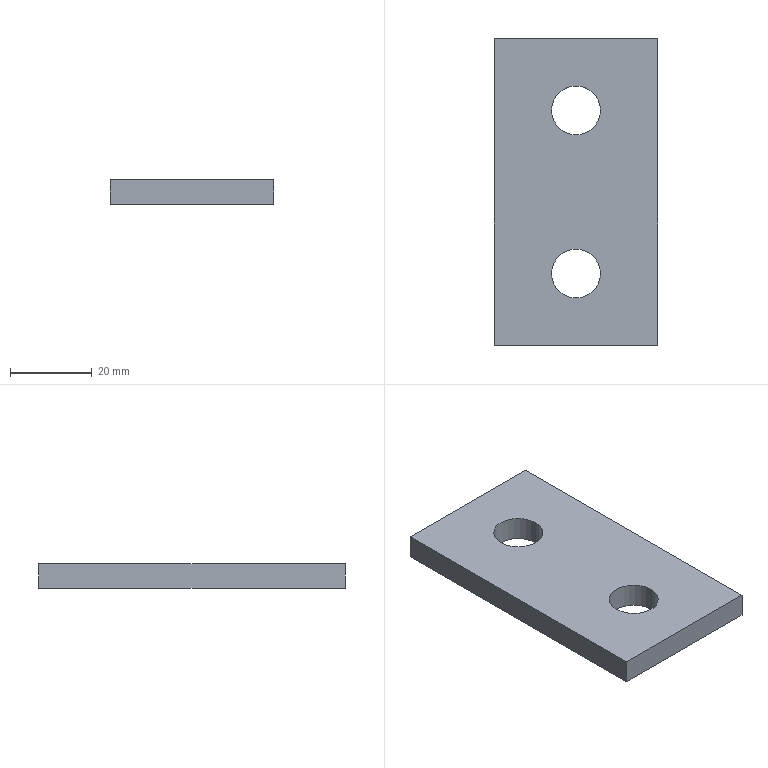Part | STEP file | BCC3 H13_10 | 1 solid | 10 faces | box 40 x 75 x 6 mm | volume 16643 mm3 | plane 6 | cylinder 4 | commonest cylinder face diameters 12 x4
STEP:
#1=CARTESIAN_POINT('',(0.,0.,0.));
#2=DIRECTION('',(0.,0.,1.));
#3=DIRECTION('',(1.,0.,0.));
#4=AXIS2_PLACEMENT_3D('',#1,#2,#3);
#5=CARTESIAN_POINT('',(6.,-20.,0.));
#6=VERTEX_POINT('',#5);
#7=CARTESIAN_POINT('',(6.,-20.,6.));
#8=VERTEX_POINT('',#7);
#9=CARTESIAN_POINT('',(6.,-20.,0.));
#10=DIRECTION('',(0.,0.,1.));
#11=VECTOR('',#10,1.);
#12=LINE('',#9,#11);
#13=CARTESIAN_POINT('',(0.,-20.,0.));
#14=DIRECTION('',(0.,0.,1.));
#15=DIRECTION('',(1.,0.,0.));
#16=AXIS2_PLACEMENT_3D('',#13,#14,#15);
#17=CYLINDRICAL_SURFACE('',#16,6.);
#18=CARTESIAN_POINT('',(6.283,0.));
#19=DIRECTION('',(0.,1.));
#20=VECTOR('',#19,1.);
#21=LINE('',#18,#20);
#22=(GEOMETRIC_REPRESENTATION_CONTEXT(2)PARAMETRIC_REPRESENTATION_CONTEXT()REPRESENTATION_CONTEXT('',''));
#23=DEFINITIONAL_REPRESENTATION('',(#21),#22);
#24=PCURVE('',#17,#23);
#25=CARTESIAN_POINT('',(0.,-20.,0.));
#26=DIRECTION('',(0.,0.,1.));
#27=DIRECTION('',(1.,0.,0.));
#28=AXIS2_PLACEMENT_3D('',#25,#26,#27);
#29=CYLINDRICAL_SURFACE('',#28,6.);
#30=CARTESIAN_POINT('',(0.,0.));
#31=DIRECTION('',(0.,1.));
#32=VECTOR('',#31,1.);
#33=LINE('',#30,#32);
#34=(GEOMETRIC_REPRESENTATION_CONTEXT(2)PARAMETRIC_REPRESENTATION_CONTEXT()REPRESENTATION_CONTEXT('',''));
#35=DEFINITIONAL_REPRESENTATION('',(#33),#34);
#36=PCURVE('',#29,#35);
#37=SURFACE_CURVE('',#12,(#24,#36),.PCURVE_S1.);
#38=EDGE_CURVE('',#6,#8,#37,.T.);
#39=ORIENTED_EDGE('',*,*,#38,.T.);
#40=CARTESIAN_POINT('',(-6.,-20.,6.));
#41=VERTEX_POINT('',#40);
#42=CARTESIAN_POINT('',(0.,-20.,6.));
#43=DIRECTION('',(0.,0.,1.));
#44=DIRECTION('',(1.,0.,0.));
#45=AXIS2_PLACEMENT_3D('',#42,#43,#44);
#46=CIRCLE('',#45,6.);
#47=CARTESIAN_POINT('',(0.,6.));
#48=DIRECTION('',(1.,0.));
#49=VECTOR('',#48,1.);
#50=LINE('',#47,#49);
#51=(GEOMETRIC_REPRESENTATION_CONTEXT(2)PARAMETRIC_REPRESENTATION_CONTEXT()REPRESENTATION_CONTEXT('',''));
#52=DEFINITIONAL_REPRESENTATION('',(#50),#51);
#53=PCURVE('',#17,#52);
#54=CARTESIAN_POINT('',(0.,0.,6.));
#55=DIRECTION('',(0.,0.,1.));
#56=DIRECTION('',(1.,0.,0.));
#57=AXIS2_PLACEMENT_3D('',#54,#55,#56);
#58=PLANE('',#57);
#59=CARTESIAN_POINT('',(0.,-20.));
#60=DIRECTION('',(1.,0.));
#61=AXIS2_PLACEMENT_2D('',#59,#60);
#62=CIRCLE('',#61,6.);
#63=(GEOMETRIC_REPRESENTATION_CONTEXT(2)PARAMETRIC_REPRESENTATION_CONTEXT()REPRESENTATION_CONTEXT('',''));
#64=DEFINITIONAL_REPRESENTATION('',(#62),#63);
#65=PCURVE('',#58,#64);
#66=SURFACE_CURVE('',#46,(#53,#65),.PCURVE_S1.);
#67=EDGE_CURVE('',#41,#8,#66,.T.);
#68=ORIENTED_EDGE('',*,*,#67,.F.);
#69=CARTESIAN_POINT('',(-6.,-20.,0.));
#70=VERTEX_POINT('',#69);
#71=CARTESIAN_POINT('',(-6.,-20.,0.));
#72=DIRECTION('',(0.,0.,1.));
#73=VECTOR('',#72,1.);
#74=LINE('',#71,#73);
#75=CARTESIAN_POINT('',(3.142,0.));
#76=DIRECTION('',(0.,1.));
#77=VECTOR('',#76,1.);
#78=LINE('',#75,#77);
#79=(GEOMETRIC_REPRESENTATION_CONTEXT(2)PARAMETRIC_REPRESENTATION_CONTEXT()REPRESENTATION_CONTEXT('',''));
#80=DEFINITIONAL_REPRESENTATION('',(#78),#79);
#81=PCURVE('',#17,#80);
#82=CARTESIAN_POINT('',(3.142,0.));
#83=DIRECTION('',(0.,1.));
#84=VECTOR('',#83,1.);
#85=LINE('',#82,#84);
#86=(GEOMETRIC_REPRESENTATION_CONTEXT(2)PARAMETRIC_REPRESENTATION_CONTEXT()REPRESENTATION_CONTEXT('',''));
#87=DEFINITIONAL_REPRESENTATION('',(#85),#86);
#88=PCURVE('',#29,#87);
#89=SURFACE_CURVE('',#74,(#81,#88),.PCURVE_S1.);
#90=EDGE_CURVE('',#70,#41,#89,.T.);
#91=ORIENTED_EDGE('',*,*,#90,.F.);
#92=CARTESIAN_POINT('',(0.,-20.,0.));
#93=DIRECTION('',(0.,0.,1.));
#94=DIRECTION('',(1.,0.,0.));
#95=AXIS2_PLACEMENT_3D('',#92,#93,#94);
#96=CIRCLE('',#95,6.);
#97=CARTESIAN_POINT('',(0.,0.));
#98=DIRECTION('',(1.,0.));
#99=VECTOR('',#98,1.);
#100=LINE('',#97,#99);
#101=(GEOMETRIC_REPRESENTATION_CONTEXT(2)PARAMETRIC_REPRESENTATION_CONTEXT()REPRESENTATION_CONTEXT('',''));
#102=DEFINITIONAL_REPRESENTATION('',(#100),#101);
#103=PCURVE('',#17,#102);
#104=CARTESIAN_POINT('',(0.,0.,0.));
#105=DIRECTION('',(0.,0.,1.));
#106=DIRECTION('',(1.,0.,0.));
#107=AXIS2_PLACEMENT_3D('',#104,#105,#106);
#108=PLANE('',#107);
#109=CARTESIAN_POINT('',(0.,-20.));
#110=DIRECTION('',(1.,0.));
#111=AXIS2_PLACEMENT_2D('',#109,#110);
#112=CIRCLE('',#111,6.);
#113=(GEOMETRIC_REPRESENTATION_CONTEXT(2)PARAMETRIC_REPRESENTATION_CONTEXT()REPRESENTATION_CONTEXT('',''));
#114=DEFINITIONAL_REPRESENTATION('',(#112),#113);
#115=PCURVE('',#108,#114);
#116=SURFACE_CURVE('',#96,(#103,#115),.PCURVE_S1.);
#117=EDGE_CURVE('',#70,#6,#116,.T.);
#118=ORIENTED_EDGE('',*,*,#117,.T.);
#119=EDGE_LOOP('',(#39,#68,#91,#118));
#120=FACE_BOUND('',#119,.F.);
#121=ADVANCED_FACE('',(#120),#17,.F.);
#122=CARTESIAN_POINT('',(6.,20.,0.));
#123=VERTEX_POINT('',#122);
#124=CARTESIAN_POINT('',(6.,20.,6.));
#125=VERTEX_POINT('',#124);
#126=CARTESIAN_POINT('',(6.,20.,0.));
#127=DIRECTION('',(0.,0.,1.));
#128=VECTOR('',#127,1.);
#129=LINE('',#126,#128);
#130=CARTESIAN_POINT('',(0.,20.,0.));
#131=DIRECTION('',(0.,0.,1.));
#132=DIRECTION('',(1.,0.,0.));
#133=AXIS2_PLACEMENT_3D('',#130,#131,#132);
#134=CYLINDRICAL_SURFACE('',#133,6.);
#135=CARTESIAN_POINT('',(6.283,0.));
#136=DIRECTION('',(0.,1.));
#137=VECTOR('',#136,1.);
#138=LINE('',#135,#137);
#139=(GEOMETRIC_REPRESENTATION_CONTEXT(2)PARAMETRIC_REPRESENTATION_CONTEXT()REPRESENTATION_CONTEXT('',''));
#140=DEFINITIONAL_REPRESENTATION('',(#138),#139);
#141=PCURVE('',#134,#140);
#142=CARTESIAN_POINT('',(0.,20.,0.));
#143=DIRECTION('',(0.,0.,1.));
#144=DIRECTION('',(1.,0.,0.));
#145=AXIS2_PLACEMENT_3D('',#142,#143,#144);
#146=CYLINDRICAL_SURFACE('',#145,6.);
#147=CARTESIAN_POINT('',(0.,0.));
#148=DIRECTION('',(0.,1.));
#149=VECTOR('',#148,1.);
#150=LINE('',#147,#149);
#151=(GEOMETRIC_REPRESENTATION_CONTEXT(2)PARAMETRIC_REPRESENTATION_CONTEXT()REPRESENTATION_CONTEXT('',''));
#152=DEFINITIONAL_REPRESENTATION('',(#150),#151);
#153=PCURVE('',#146,#152);
#154=SURFACE_CURVE('',#129,(#141,#153),.PCURVE_S1.);
#155=EDGE_CURVE('',#123,#125,#154,.T.);
#156=ORIENTED_EDGE('',*,*,#155,.T.);
#157=CARTESIAN_POINT('',(-6.,20.,6.));
#158=VERTEX_POINT('',#157);
#159=CARTESIAN_POINT('',(0.,20.,6.));
#160=DIRECTION('',(0.,0.,1.));
#161=DIRECTION('',(1.,0.,0.));
#162=AXIS2_PLACEMENT_3D('',#159,#160,#161);
#163=CIRCLE('',#162,6.);
#164=CARTESIAN_POINT('',(0.,6.));
#165=DIRECTION('',(1.,0.));
#166=VECTOR('',#165,1.);
#167=LINE('',#164,#166);
#168=(GEOMETRIC_REPRESENTATION_CONTEXT(2)PARAMETRIC_REPRESENTATION_CONTEXT()REPRESENTATION_CONTEXT('',''));
#169=DEFINITIONAL_REPRESENTATION('',(#167),#168);
#170=PCURVE('',#134,#169);
#171=CARTESIAN_POINT('',(0.,20.));
#172=DIRECTION('',(1.,0.));
#173=AXIS2_PLACEMENT_2D('',#171,#172);
#174=CIRCLE('',#173,6.);
#175=(GEOMETRIC_REPRESENTATION_CONTEXT(2)PARAMETRIC_REPRESENTATION_CONTEXT()REPRESENTATION_CONTEXT('',''));
#176=DEFINITIONAL_REPRESENTATION('',(#174),#175);
#177=PCURVE('',#58,#176);
#178=SURFACE_CURVE('',#163,(#170,#177),.PCURVE_S1.);
#179=EDGE_CURVE('',#158,#125,#178,.T.);
#180=ORIENTED_EDGE('',*,*,#179,.F.);
#181=CARTESIAN_POINT('',(-6.,20.,0.));
#182=VERTEX_POINT('',#181);
#183=CARTESIAN_POINT('',(-6.,20.,0.));
#184=DIRECTION('',(0.,0.,1.));
#185=VECTOR('',#184,1.);
#186=LINE('',#183,#185);
#187=CARTESIAN_POINT('',(3.142,0.));
#188=DIRECTION('',(0.,1.));
#189=VECTOR('',#188,1.);
#190=LINE('',#187,#189);
#191=(GEOMETRIC_REPRESENTATION_CONTEXT(2)PARAMETRIC_REPRESENTATION_CONTEXT()REPRESENTATION_CONTEXT('',''));
#192=DEFINITIONAL_REPRESENTATION('',(#190),#191);
#193=PCURVE('',#134,#192);
#194=CARTESIAN_POINT('',(3.142,0.));
#195=DIRECTION('',(0.,1.));
#196=VECTOR('',#195,1.);
#197=LINE('',#194,#196);
#198=(GEOMETRIC_REPRESENTATION_CONTEXT(2)PARAMETRIC_REPRESENTATION_CONTEXT()REPRESENTATION_CONTEXT('',''));
#199=DEFINITIONAL_REPRESENTATION('',(#197),#198);
#200=PCURVE('',#146,#199);
#201=SURFACE_CURVE('',#186,(#193,#200),.PCURVE_S1.);
#202=EDGE_CURVE('',#182,#158,#201,.T.);
#203=ORIENTED_EDGE('',*,*,#202,.F.);
#204=CARTESIAN_POINT('',(0.,20.,0.));
#205=DIRECTION('',(0.,0.,1.));
#206=DIRECTION('',(1.,0.,0.));
#207=AXIS2_PLACEMENT_3D('',#204,#205,#206);
#208=CIRCLE('',#207,6.);
#209=CARTESIAN_POINT('',(0.,0.));
#210=DIRECTION('',(1.,0.));
#211=VECTOR('',#210,1.);
#212=LINE('',#209,#211);
#213=(GEOMETRIC_REPRESENTATION_CONTEXT(2)PARAMETRIC_REPRESENTATION_CONTEXT()REPRESENTATION_CONTEXT('',''));
#214=DEFINITIONAL_REPRESENTATION('',(#212),#213);
#215=PCURVE('',#134,#214);
#216=CARTESIAN_POINT('',(0.,20.));
#217=DIRECTION('',(1.,0.));
#218=AXIS2_PLACEMENT_2D('',#216,#217);
#219=CIRCLE('',#218,6.);
#220=(GEOMETRIC_REPRESENTATION_CONTEXT(2)PARAMETRIC_REPRESENTATION_CONTEXT()REPRESENTATION_CONTEXT('',''));
#221=DEFINITIONAL_REPRESENTATION('',(#219),#220);
#222=PCURVE('',#108,#221);
#223=SURFACE_CURVE('',#208,(#215,#222),.PCURVE_S1.);
#224=EDGE_CURVE('',#182,#123,#223,.T.);
#225=ORIENTED_EDGE('',*,*,#224,.T.);
#226=EDGE_LOOP('',(#156,#180,#203,#225));
#227=FACE_BOUND('',#226,.F.);
#228=ADVANCED_FACE('',(#227),#134,.F.);
#229=CARTESIAN_POINT('',(-20.,37.5,0.));
#230=VERTEX_POINT('',#229);
#231=CARTESIAN_POINT('',(-20.,-37.5,0.));
#232=VERTEX_POINT('',#231);
#233=CARTESIAN_POINT('',(-20.,37.5,0.));
#234=DIRECTION('',(0.,-1.,0.));
#235=VECTOR('',#234,1.);
#236=LINE('',#233,#235);
#237=CARTESIAN_POINT('',(-20.,37.5,6.));
#238=DIRECTION('',(1.,0.,0.));
#239=DIRECTION('',(0.,1.,0.));
#240=AXIS2_PLACEMENT_3D('',#237,#238,#239);
#241=PLANE('',#240);
#242=CARTESIAN_POINT('',(0.,-6.));
#243=DIRECTION('',(-1.,0.));
#244=VECTOR('',#243,1.);
#245=LINE('',#242,#244);
#246=(GEOMETRIC_REPRESENTATION_CONTEXT(2)PARAMETRIC_REPRESENTATION_CONTEXT()REPRESENTATION_CONTEXT('',''));
#247=DEFINITIONAL_REPRESENTATION('',(#245),#246);
#248=PCURVE('',#241,#247);
#249=CARTESIAN_POINT('',(-20.,37.5));
#250=DIRECTION('',(0.,-1.));
#251=VECTOR('',#250,1.);
#252=LINE('',#249,#251);
#253=(GEOMETRIC_REPRESENTATION_CONTEXT(2)PARAMETRIC_REPRESENTATION_CONTEXT()REPRESENTATION_CONTEXT('',''));
#254=DEFINITIONAL_REPRESENTATION('',(#252),#253);
#255=PCURVE('',#108,#254);
#256=SURFACE_CURVE('',#236,(#248,#255),.PCURVE_S1.);
#257=EDGE_CURVE('',#230,#232,#256,.T.);
#258=ORIENTED_EDGE('',*,*,#257,.T.);
#259=CARTESIAN_POINT('',(-20.,-37.5,6.));
#260=VERTEX_POINT('',#259);
#261=CARTESIAN_POINT('',(-20.,-37.5,6.));
#262=DIRECTION('',(0.,0.,-1.));
#263=VECTOR('',#262,1.);
#264=LINE('',#261,#263);
#265=CARTESIAN_POINT('',(-75.,0.));
#266=DIRECTION('',(0.,-1.));
#267=VECTOR('',#266,1.);
#268=LINE('',#265,#267);
#269=(GEOMETRIC_REPRESENTATION_CONTEXT(2)PARAMETRIC_REPRESENTATION_CONTEXT()REPRESENTATION_CONTEXT('',''));
#270=DEFINITIONAL_REPRESENTATION('',(#268),#269);
#271=PCURVE('',#241,#270);
#272=CARTESIAN_POINT('',(-20.,-37.5,6.));
#273=DIRECTION('',(0.,1.,0.));
#274=DIRECTION('',(0.,0.,1.));
#275=AXIS2_PLACEMENT_3D('',#272,#273,#274);
#276=PLANE('',#275);
#277=CARTESIAN_POINT('',(0.,0.));
#278=DIRECTION('',(-1.,0.));
#279=VECTOR('',#278,1.);
#280=LINE('',#277,#279);
#281=(GEOMETRIC_REPRESENTATION_CONTEXT(2)PARAMETRIC_REPRESENTATION_CONTEXT()REPRESENTATION_CONTEXT('',''));
#282=DEFINITIONAL_REPRESENTATION('',(#280),#281);
#283=PCURVE('',#276,#282);
#284=SURFACE_CURVE('',#264,(#271,#283),.PCURVE_S1.);
#285=EDGE_CURVE('',#260,#232,#284,.T.);
#286=ORIENTED_EDGE('',*,*,#285,.F.);
#287=CARTESIAN_POINT('',(-20.,37.5,6.));
#288=VERTEX_POINT('',#287);
#289=CARTESIAN_POINT('',(-20.,37.5,6.));
#290=DIRECTION('',(0.,-1.,0.));
#291=VECTOR('',#290,1.);
#292=LINE('',#289,#291);
#293=CARTESIAN_POINT('',(0.,0.));
#294=DIRECTION('',(-1.,0.));
#295=VECTOR('',#294,1.);
#296=LINE('',#293,#295);
#297=(GEOMETRIC_REPRESENTATION_CONTEXT(2)PARAMETRIC_REPRESENTATION_CONTEXT()REPRESENTATION_CONTEXT('',''));
#298=DEFINITIONAL_REPRESENTATION('',(#296),#297);
#299=PCURVE('',#241,#298);
#300=CARTESIAN_POINT('',(-20.,37.5));
#301=DIRECTION('',(0.,-1.));
#302=VECTOR('',#301,1.);
#303=LINE('',#300,#302);
#304=(GEOMETRIC_REPRESENTATION_CONTEXT(2)PARAMETRIC_REPRESENTATION_CONTEXT()REPRESENTATION_CONTEXT('',''));
#305=DEFINITIONAL_REPRESENTATION('',(#303),#304);
#306=PCURVE('',#58,#305);
#307=SURFACE_CURVE('',#292,(#299,#306),.PCURVE_S1.);
#308=EDGE_CURVE('',#288,#260,#307,.T.);
#309=ORIENTED_EDGE('',*,*,#308,.F.);
#310=CARTESIAN_POINT('',(-20.,37.5,6.));
#311=DIRECTION('',(0.,0.,-1.));
#312=VECTOR('',#311,1.);
#313=LINE('',#310,#312);
#314=CARTESIAN_POINT('',(0.,0.));
#315=DIRECTION('',(0.,-1.));
#316=VECTOR('',#315,1.);
#317=LINE('',#314,#316);
#318=(GEOMETRIC_REPRESENTATION_CONTEXT(2)PARAMETRIC_REPRESENTATION_CONTEXT()REPRESENTATION_CONTEXT('',''));
#319=DEFINITIONAL_REPRESENTATION('',(#317),#318);
#320=PCURVE('',#241,#319);
#321=CARTESIAN_POINT('',(-20.,37.5,6.));
#322=DIRECTION('',(0.,-1.,0.));
#323=DIRECTION('',(0.,0.,-1.));
#324=AXIS2_PLACEMENT_3D('',#321,#322,#323);
#325=PLANE('',#324);
#326=CARTESIAN_POINT('',(0.,0.));
#327=DIRECTION('',(1.,0.));
#328=VECTOR('',#327,1.);
#329=LINE('',#326,#328);
#330=(GEOMETRIC_REPRESENTATION_CONTEXT(2)PARAMETRIC_REPRESENTATION_CONTEXT()REPRESENTATION_CONTEXT('',''));
#331=DEFINITIONAL_REPRESENTATION('',(#329),#330);
#332=PCURVE('',#325,#331);
#333=SURFACE_CURVE('',#313,(#320,#332),.PCURVE_S1.);
#334=EDGE_CURVE('',#288,#230,#333,.T.);
#335=ORIENTED_EDGE('',*,*,#334,.T.);
#336=EDGE_LOOP('',(#258,#286,#309,#335));
#337=FACE_BOUND('',#336,.T.);
#338=ADVANCED_FACE('',(#337),#241,.F.);
#339=CARTESIAN_POINT('',(20.,-37.5,0.));
#340=VERTEX_POINT('',#339);
#341=CARTESIAN_POINT('',(-20.,-37.5,0.));
#342=DIRECTION('',(1.,0.,0.));
#343=VECTOR('',#342,1.);
#344=LINE('',#341,#343);
#345=CARTESIAN_POINT('',(-6.,0.));
#346=DIRECTION('',(0.,1.));
#347=VECTOR('',#346,1.);
#348=LINE('',#345,#347);
#349=(GEOMETRIC_REPRESENTATION_CONTEXT(2)PARAMETRIC_REPRESENTATION_CONTEXT()REPRESENTATION_CONTEXT('',''));
#350=DEFINITIONAL_REPRESENTATION('',(#348),#349);
#351=PCURVE('',#276,#350);
#352=CARTESIAN_POINT('',(-20.,-37.5));
#353=DIRECTION('',(1.,0.));
#354=VECTOR('',#353,1.);
#355=LINE('',#352,#354);
#356=(GEOMETRIC_REPRESENTATION_CONTEXT(2)PARAMETRIC_REPRESENTATION_CONTEXT()REPRESENTATION_CONTEXT('',''));
#357=DEFINITIONAL_REPRESENTATION('',(#355),#356);
#358=PCURVE('',#108,#357);
#359=SURFACE_CURVE('',#344,(#351,#358),.PCURVE_S1.);
#360=EDGE_CURVE('',#232,#340,#359,.T.);
#361=ORIENTED_EDGE('',*,*,#360,.T.);
#362=CARTESIAN_POINT('',(20.,-37.5,6.));
#363=VERTEX_POINT('',#362);
#364=CARTESIAN_POINT('',(20.,-37.5,6.));
#365=DIRECTION('',(0.,0.,-1.));
#366=VECTOR('',#365,1.);
#367=LINE('',#364,#366);
#368=CARTESIAN_POINT('',(0.,40.));
#369=DIRECTION('',(-1.,0.));
#370=VECTOR('',#369,1.);
#371=LINE('',#368,#370);
#372=(GEOMETRIC_REPRESENTATION_CONTEXT(2)PARAMETRIC_REPRESENTATION_CONTEXT()REPRESENTATION_CONTEXT('',''));
#373=DEFINITIONAL_REPRESENTATION('',(#371),#372);
#374=PCURVE('',#276,#373);
#375=CARTESIAN_POINT('',(20.,37.5,6.));
#376=DIRECTION('',(-1.,0.,0.));
#377=DIRECTION('',(0.,-1.,0.));
#378=AXIS2_PLACEMENT_3D('',#375,#376,#377);
#379=PLANE('',#378);
#380=CARTESIAN_POINT('',(75.,0.));
#381=DIRECTION('',(0.,-1.));
#382=VECTOR('',#381,1.);
#383=LINE('',#380,#382);
#384=(GEOMETRIC_REPRESENTATION_CONTEXT(2)PARAMETRIC_REPRESENTATION_CONTEXT()REPRESENTATION_CONTEXT('',''));
#385=DEFINITIONAL_REPRESENTATION('',(#383),#384);
#386=PCURVE('',#379,#385);
#387=SURFACE_CURVE('',#367,(#374,#386),.PCURVE_S1.);
#388=EDGE_CURVE('',#363,#340,#387,.T.);
#389=ORIENTED_EDGE('',*,*,#388,.F.);
#390=CARTESIAN_POINT('',(-20.,-37.5,6.));
#391=DIRECTION('',(1.,0.,0.));
#392=VECTOR('',#391,1.);
#393=LINE('',#390,#392);
#394=CARTESIAN_POINT('',(0.,0.));
#395=DIRECTION('',(0.,1.));
#396=VECTOR('',#395,1.);
#397=LINE('',#394,#396);
#398=(GEOMETRIC_REPRESENTATION_CONTEXT(2)PARAMETRIC_REPRESENTATION_CONTEXT()REPRESENTATION_CONTEXT('',''));
#399=DEFINITIONAL_REPRESENTATION('',(#397),#398);
#400=PCURVE('',#276,#399);
#401=CARTESIAN_POINT('',(-20.,-37.5));
#402=DIRECTION('',(1.,0.));
#403=VECTOR('',#402,1.);
#404=LINE('',#401,#403);
#405=(GEOMETRIC_REPRESENTATION_CONTEXT(2)PARAMETRIC_REPRESENTATION_CONTEXT()REPRESENTATION_CONTEXT('',''));
#406=DEFINITIONAL_REPRESENTATION('',(#404),#405);
#407=PCURVE('',#58,#406);
#408=SURFACE_CURVE('',#393,(#400,#407),.PCURVE_S1.);
#409=EDGE_CURVE('',#260,#363,#408,.T.);
#410=ORIENTED_EDGE('',*,*,#409,.F.);
#411=ORIENTED_EDGE('',*,*,#285,.T.);
#412=EDGE_LOOP('',(#361,#389,#410,#411));
#413=FACE_BOUND('',#412,.T.);
#414=ADVANCED_FACE('',(#413),#276,.F.);
#415=CARTESIAN_POINT('',(20.,37.5,0.));
#416=VERTEX_POINT('',#415);
#417=CARTESIAN_POINT('',(20.,37.5,0.));
#418=DIRECTION('',(0.,1.,0.));
#419=VECTOR('',#418,1.);
#420=LINE('',#417,#419);
#421=CARTESIAN_POINT('',(0.,-6.));
#422=DIRECTION('',(-1.,0.));
#423=VECTOR('',#422,1.);
#424=LINE('',#421,#423);
#425=(GEOMETRIC_REPRESENTATION_CONTEXT(2)PARAMETRIC_REPRESENTATION_CONTEXT()REPRESENTATION_CONTEXT('',''));
#426=DEFINITIONAL_REPRESENTATION('',(#424),#425);
#427=PCURVE('',#379,#426);
#428=CARTESIAN_POINT('',(20.,37.5));
#429=DIRECTION('',(0.,1.));
#430=VECTOR('',#429,1.);
#431=LINE('',#428,#430);
#432=(GEOMETRIC_REPRESENTATION_CONTEXT(2)PARAMETRIC_REPRESENTATION_CONTEXT()REPRESENTATION_CONTEXT('',''));
#433=DEFINITIONAL_REPRESENTATION('',(#431),#432);
#434=PCURVE('',#108,#433);
#435=SURFACE_CURVE('',#420,(#427,#434),.PCURVE_S1.);
#436=EDGE_CURVE('',#340,#416,#435,.T.);
#437=ORIENTED_EDGE('',*,*,#436,.T.);
#438=CARTESIAN_POINT('',(20.,37.5,6.));
#439=VERTEX_POINT('',#438);
#440=CARTESIAN_POINT('',(20.,37.5,6.));
#441=DIRECTION('',(0.,0.,-1.));
#442=VECTOR('',#441,1.);
#443=LINE('',#440,#442);
#444=CARTESIAN_POINT('',(0.,0.));
#445=DIRECTION('',(0.,-1.));
#446=VECTOR('',#445,1.);
#447=LINE('',#444,#446);
#448=(GEOMETRIC_REPRESENTATION_CONTEXT(2)PARAMETRIC_REPRESENTATION_CONTEXT()REPRESENTATION_CONTEXT('',''));
#449=DEFINITIONAL_REPRESENTATION('',(#447),#448);
#450=PCURVE('',#379,#449);
#451=CARTESIAN_POINT('',(0.,40.));
#452=DIRECTION('',(1.,0.));
#453=VECTOR('',#452,1.);
#454=LINE('',#451,#453);
#455=(GEOMETRIC_REPRESENTATION_CONTEXT(2)PARAMETRIC_REPRESENTATION_CONTEXT()REPRESENTATION_CONTEXT('',''));
#456=DEFINITIONAL_REPRESENTATION('',(#454),#455);
#457=PCURVE('',#325,#456);
#458=SURFACE_CURVE('',#443,(#450,#457),.PCURVE_S1.);
#459=EDGE_CURVE('',#439,#416,#458,.T.);
#460=ORIENTED_EDGE('',*,*,#459,.F.);
#461=CARTESIAN_POINT('',(20.,37.5,6.));
#462=DIRECTION('',(0.,1.,0.));
#463=VECTOR('',#462,1.);
#464=LINE('',#461,#463);
#465=CARTESIAN_POINT('',(0.,0.));
#466=DIRECTION('',(-1.,0.));
#467=VECTOR('',#466,1.);
#468=LINE('',#465,#467);
#469=(GEOMETRIC_REPRESENTATION_CONTEXT(2)PARAMETRIC_REPRESENTATION_CONTEXT()REPRESENTATION_CONTEXT('',''));
#470=DEFINITIONAL_REPRESENTATION('',(#468),#469);
#471=PCURVE('',#379,#470);
#472=CARTESIAN_POINT('',(20.,37.5));
#473=DIRECTION('',(0.,1.));
#474=VECTOR('',#473,1.);
#475=LINE('',#472,#474);
#476=(GEOMETRIC_REPRESENTATION_CONTEXT(2)PARAMETRIC_REPRESENTATION_CONTEXT()REPRESENTATION_CONTEXT('',''));
#477=DEFINITIONAL_REPRESENTATION('',(#475),#476);
#478=PCURVE('',#58,#477);
#479=SURFACE_CURVE('',#464,(#471,#478),.PCURVE_S1.);
#480=EDGE_CURVE('',#363,#439,#479,.T.);
#481=ORIENTED_EDGE('',*,*,#480,.F.);
#482=ORIENTED_EDGE('',*,*,#388,.T.);
#483=EDGE_LOOP('',(#437,#460,#481,#482));
#484=FACE_BOUND('',#483,.T.);
#485=ADVANCED_FACE('',(#484),#379,.F.);
#486=CARTESIAN_POINT('',(-20.,37.5,0.));
#487=DIRECTION('',(-1.,0.,0.));
#488=VECTOR('',#487,1.);
#489=LINE('',#486,#488);
#490=CARTESIAN_POINT('',(6.,0.));
#491=DIRECTION('',(0.,-1.));
#492=VECTOR('',#491,1.);
#493=LINE('',#490,#492);
#494=(GEOMETRIC_REPRESENTATION_CONTEXT(2)PARAMETRIC_REPRESENTATION_CONTEXT()REPRESENTATION_CONTEXT('',''));
#495=DEFINITIONAL_REPRESENTATION('',(#493),#494);
#496=PCURVE('',#325,#495);
#497=CARTESIAN_POINT('',(-20.,37.5));
#498=DIRECTION('',(-1.,0.));
#499=VECTOR('',#498,1.);
#500=LINE('',#497,#499);
#501=(GEOMETRIC_REPRESENTATION_CONTEXT(2)PARAMETRIC_REPRESENTATION_CONTEXT()REPRESENTATION_CONTEXT('',''));
#502=DEFINITIONAL_REPRESENTATION('',(#500),#501);
#503=PCURVE('',#108,#502);
#504=SURFACE_CURVE('',#489,(#496,#503),.PCURVE_S1.);
#505=EDGE_CURVE('',#416,#230,#504,.T.);
#506=ORIENTED_EDGE('',*,*,#505,.T.);
#507=ORIENTED_EDGE('',*,*,#334,.F.);
#508=CARTESIAN_POINT('',(-20.,37.5,6.));
#509=DIRECTION('',(-1.,0.,0.));
#510=VECTOR('',#509,1.);
#511=LINE('',#508,#510);
#512=CARTESIAN_POINT('',(0.,0.));
#513=DIRECTION('',(0.,-1.));
#514=VECTOR('',#513,1.);
#515=LINE('',#512,#514);
#516=(GEOMETRIC_REPRESENTATION_CONTEXT(2)PARAMETRIC_REPRESENTATION_CONTEXT()REPRESENTATION_CONTEXT('',''));
#517=DEFINITIONAL_REPRESENTATION('',(#515),#516);
#518=PCURVE('',#325,#517);
#519=CARTESIAN_POINT('',(-20.,37.5));
#520=DIRECTION('',(-1.,0.));
#521=VECTOR('',#520,1.);
#522=LINE('',#519,#521);
#523=(GEOMETRIC_REPRESENTATION_CONTEXT(2)PARAMETRIC_REPRESENTATION_CONTEXT()REPRESENTATION_CONTEXT('',''));
#524=DEFINITIONAL_REPRESENTATION('',(#522),#523);
#525=PCURVE('',#58,#524);
#526=SURFACE_CURVE('',#511,(#518,#525),.PCURVE_S1.);
#527=EDGE_CURVE('',#439,#288,#526,.T.);
#528=ORIENTED_EDGE('',*,*,#527,.F.);
#529=ORIENTED_EDGE('',*,*,#459,.T.);
#530=EDGE_LOOP('',(#506,#507,#528,#529));
#531=FACE_BOUND('',#530,.T.);
#532=ADVANCED_FACE('',(#531),#325,.F.);
#533=CARTESIAN_POINT('',(0.,-20.,6.));
#534=DIRECTION('',(0.,0.,1.));
#535=DIRECTION('',(1.,0.,0.));
#536=AXIS2_PLACEMENT_3D('',#533,#534,#535);
#537=CIRCLE('',#536,6.);
#538=CARTESIAN_POINT('',(0.,-20.));
#539=DIRECTION('',(1.,0.));
#540=AXIS2_PLACEMENT_2D('',#538,#539);
#541=CIRCLE('',#540,6.);
#542=(GEOMETRIC_REPRESENTATION_CONTEXT(2)PARAMETRIC_REPRESENTATION_CONTEXT()REPRESENTATION_CONTEXT('',''));
#543=DEFINITIONAL_REPRESENTATION('',(#541),#542);
#544=PCURVE('',#58,#543);
#545=CARTESIAN_POINT('',(0.,6.));
#546=DIRECTION('',(1.,0.));
#547=VECTOR('',#546,1.);
#548=LINE('',#545,#547);
#549=(GEOMETRIC_REPRESENTATION_CONTEXT(2)PARAMETRIC_REPRESENTATION_CONTEXT()REPRESENTATION_CONTEXT('',''));
#550=DEFINITIONAL_REPRESENTATION('',(#548),#549);
#551=PCURVE('',#29,#550);
#552=SURFACE_CURVE('',#537,(#544,#551),.PCURVE_S1.);
#553=EDGE_CURVE('',#8,#41,#552,.T.);
#554=ORIENTED_EDGE('',*,*,#553,.F.);
#555=ORIENTED_EDGE('',*,*,#67,.F.);
#556=EDGE_LOOP('',(#554,#555));
#557=FACE_BOUND('',#556,.T.);
#558=CARTESIAN_POINT('',(0.,20.,6.));
#559=DIRECTION('',(0.,0.,1.));
#560=DIRECTION('',(1.,0.,0.));
#561=AXIS2_PLACEMENT_3D('',#558,#559,#560);
#562=CIRCLE('',#561,6.);
#563=CARTESIAN_POINT('',(0.,20.));
#564=DIRECTION('',(1.,0.));
#565=AXIS2_PLACEMENT_2D('',#563,#564);
#566=CIRCLE('',#565,6.);
#567=(GEOMETRIC_REPRESENTATION_CONTEXT(2)PARAMETRIC_REPRESENTATION_CONTEXT()REPRESENTATION_CONTEXT('',''));
#568=DEFINITIONAL_REPRESENTATION('',(#566),#567);
#569=PCURVE('',#58,#568);
#570=CARTESIAN_POINT('',(0.,6.));
#571=DIRECTION('',(1.,0.));
#572=VECTOR('',#571,1.);
#573=LINE('',#570,#572);
#574=(GEOMETRIC_REPRESENTATION_CONTEXT(2)PARAMETRIC_REPRESENTATION_CONTEXT()REPRESENTATION_CONTEXT('',''));
#575=DEFINITIONAL_REPRESENTATION('',(#573),#574);
#576=PCURVE('',#146,#575);
#577=SURFACE_CURVE('',#562,(#569,#576),.PCURVE_S1.);
#578=EDGE_CURVE('',#125,#158,#577,.T.);
#579=ORIENTED_EDGE('',*,*,#578,.F.);
#580=ORIENTED_EDGE('',*,*,#179,.F.);
#581=EDGE_LOOP('',(#579,#580));
#582=FACE_BOUND('',#581,.T.);
#583=ORIENTED_EDGE('',*,*,#308,.T.);
#584=ORIENTED_EDGE('',*,*,#409,.T.);
#585=ORIENTED_EDGE('',*,*,#480,.T.);
#586=ORIENTED_EDGE('',*,*,#527,.T.);
#587=EDGE_LOOP('',(#583,#584,#585,#586));
#588=FACE_BOUND('',#587,.T.);
#589=ADVANCED_FACE('',(#557,#582,#588),#58,.T.);
#590=CARTESIAN_POINT('',(0.,-20.,0.));
#591=DIRECTION('',(0.,0.,1.));
#592=DIRECTION('',(1.,0.,0.));
#593=AXIS2_PLACEMENT_3D('',#590,#591,#592);
#594=CIRCLE('',#593,6.);
#595=CARTESIAN_POINT('',(0.,-20.));
#596=DIRECTION('',(1.,0.));
#597=AXIS2_PLACEMENT_2D('',#595,#596);
#598=CIRCLE('',#597,6.);
#599=(GEOMETRIC_REPRESENTATION_CONTEXT(2)PARAMETRIC_REPRESENTATION_CONTEXT()REPRESENTATION_CONTEXT('',''));
#600=DEFINITIONAL_REPRESENTATION('',(#598),#599);
#601=PCURVE('',#108,#600);
#602=CARTESIAN_POINT('',(0.,0.));
#603=DIRECTION('',(1.,0.));
#604=VECTOR('',#603,1.);
#605=LINE('',#602,#604);
#606=(GEOMETRIC_REPRESENTATION_CONTEXT(2)PARAMETRIC_REPRESENTATION_CONTEXT()REPRESENTATION_CONTEXT('',''));
#607=DEFINITIONAL_REPRESENTATION('',(#605),#606);
#608=PCURVE('',#29,#607);
#609=SURFACE_CURVE('',#594,(#601,#608),.PCURVE_S1.);
#610=EDGE_CURVE('',#6,#70,#609,.T.);
#611=ORIENTED_EDGE('',*,*,#610,.T.);
#612=ORIENTED_EDGE('',*,*,#117,.T.);
#613=EDGE_LOOP('',(#611,#612));
#614=FACE_BOUND('',#613,.T.);
#615=CARTESIAN_POINT('',(0.,20.,0.));
#616=DIRECTION('',(0.,0.,1.));
#617=DIRECTION('',(1.,0.,0.));
#618=AXIS2_PLACEMENT_3D('',#615,#616,#617);
#619=CIRCLE('',#618,6.);
#620=CARTESIAN_POINT('',(0.,20.));
#621=DIRECTION('',(1.,0.));
#622=AXIS2_PLACEMENT_2D('',#620,#621);
#623=CIRCLE('',#622,6.);
#624=(GEOMETRIC_REPRESENTATION_CONTEXT(2)PARAMETRIC_REPRESENTATION_CONTEXT()REPRESENTATION_CONTEXT('',''));
#625=DEFINITIONAL_REPRESENTATION('',(#623),#624);
#626=PCURVE('',#108,#625);
#627=CARTESIAN_POINT('',(0.,0.));
#628=DIRECTION('',(1.,0.));
#629=VECTOR('',#628,1.);
#630=LINE('',#627,#629);
#631=(GEOMETRIC_REPRESENTATION_CONTEXT(2)PARAMETRIC_REPRESENTATION_CONTEXT()REPRESENTATION_CONTEXT('',''));
#632=DEFINITIONAL_REPRESENTATION('',(#630),#631);
#633=PCURVE('',#146,#632);
#634=SURFACE_CURVE('',#619,(#626,#633),.PCURVE_S1.);
#635=EDGE_CURVE('',#123,#182,#634,.T.);
#636=ORIENTED_EDGE('',*,*,#635,.T.);
#637=ORIENTED_EDGE('',*,*,#224,.T.);
#638=EDGE_LOOP('',(#636,#637));
#639=FACE_BOUND('',#638,.T.);
#640=ORIENTED_EDGE('',*,*,#257,.F.);
#641=ORIENTED_EDGE('',*,*,#505,.F.);
#642=ORIENTED_EDGE('',*,*,#436,.F.);
#643=ORIENTED_EDGE('',*,*,#360,.F.);
#644=EDGE_LOOP('',(#640,#641,#642,#643));
#645=FACE_BOUND('',#644,.T.);
#646=ADVANCED_FACE('',(#614,#639,#645),#108,.F.);
#647=ORIENTED_EDGE('',*,*,#578,.F.);
#648=ORIENTED_EDGE('',*,*,#155,.F.);
#649=ORIENTED_EDGE('',*,*,#635,.T.);
#650=ORIENTED_EDGE('',*,*,#202,.T.);
#651=EDGE_LOOP('',(#647,#648,#649,#650));
#652=FACE_BOUND('',#651,.F.);
#653=ADVANCED_FACE('',(#652),#146,.F.);
#654=ORIENTED_EDGE('',*,*,#553,.F.);
#655=ORIENTED_EDGE('',*,*,#38,.F.);
#656=ORIENTED_EDGE('',*,*,#610,.T.);
#657=ORIENTED_EDGE('',*,*,#90,.T.);
#658=EDGE_LOOP('',(#654,#655,#656,#657));
#659=FACE_BOUND('',#658,.F.);
#660=ADVANCED_FACE('',(#659),#29,.F.);
#661=CLOSED_SHELL('',(#121,#228,#338,#414,#485,#532,#589,#646,#653,#660));
#662=MANIFOLD_SOLID_BREP('',#661);
#663=(LENGTH_UNIT()NAMED_UNIT(*)SI_UNIT(.MILLI.,.METRE.));
#664=UNCERTAINTY_MEASURE_WITH_UNIT(LENGTH_MEASURE(0.0000001),#663,'','');
#665=(NAMED_UNIT(*)PLANE_ANGLE_UNIT()SI_UNIT($,.RADIAN.));
#666=(NAMED_UNIT(*)SI_UNIT($,.STERADIAN.)SOLID_ANGLE_UNIT());
#667=(GEOMETRIC_REPRESENTATION_CONTEXT(3)GLOBAL_UNCERTAINTY_ASSIGNED_CONTEXT((#664))GLOBAL_UNIT_ASSIGNED_CONTEXT((#663,#665,#666))REPRESENTATION_CONTEXT('',''));
#668=ADVANCED_BREP_SHAPE_REPRESENTATION('',(#4,#662),#667);